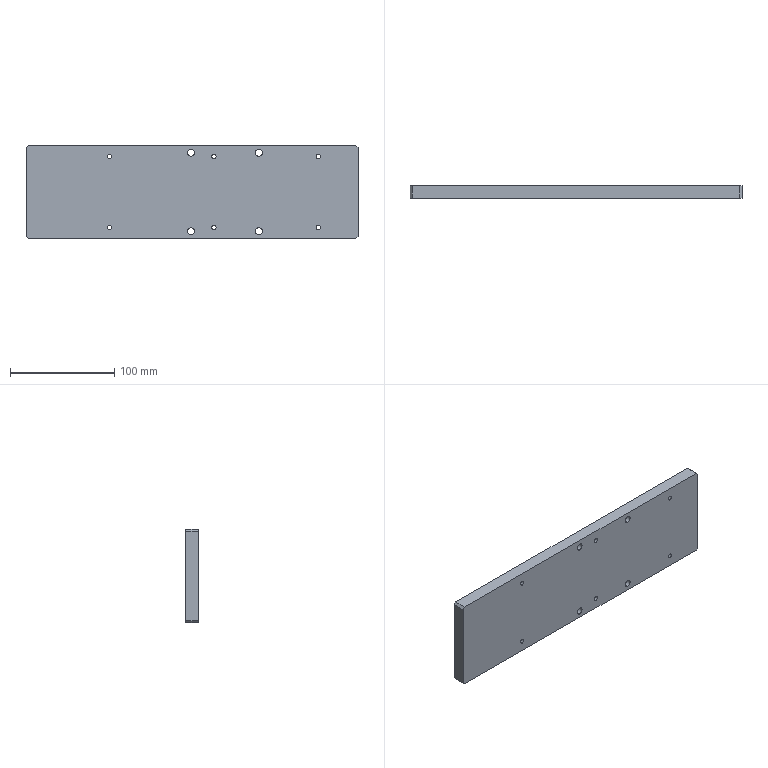Part | SolidWorks | features HoleWzd 4, Chamfer 1, Extrusion 1 | 1 solid | 58 faces | box 318 x 12 x 90 mm | volume 338579 mm3 | cylinder 36 | plane 14 | cone 8 | commonest cylinder face diameters 4.2 x12 5 x8 6.6 x8 11 x8